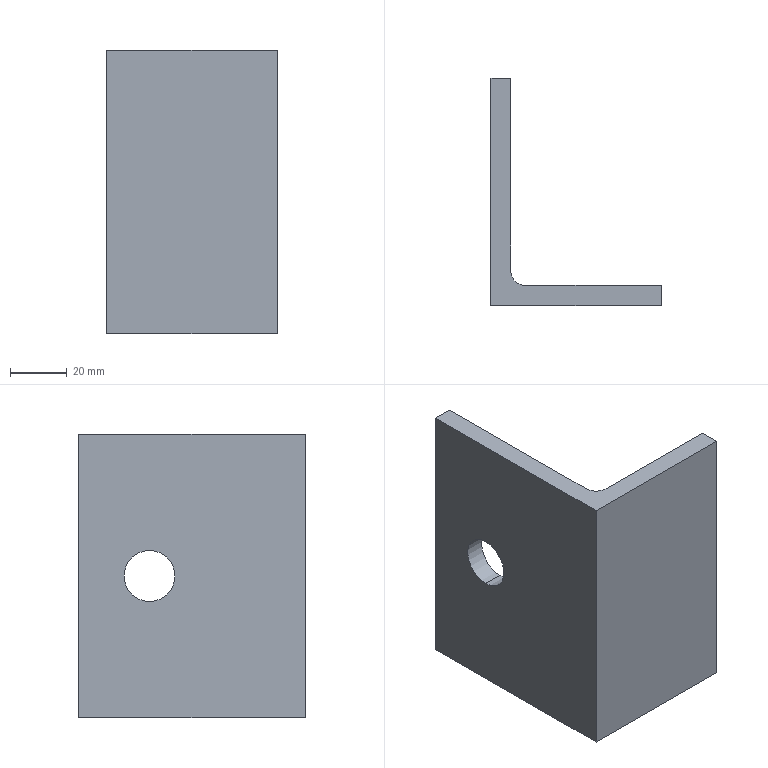Part | SolidWorks | features Extrusion 1, Fillet 1, ICE 1 | 1 solid | 11 faces | box 60 x 80 x 100 mm | volume 91855 mm3 | plane 8 | cylinder 3 | commonest cylinder face diameters 18 x2 10 x1
STEP:
#1=CARTESIAN_POINT('',(0.,-25.,59.));
#2=VERTEX_POINT('',#1);
#3=CARTESIAN_POINT('',(0.,-25.,41.));
#4=VERTEX_POINT('',#3);
#5=CARTESIAN_POINT('',(0.,-25.,50.));
#6=DIRECTION('',(1.,0.,0.));
#7=DIRECTION('',(0.,1.,0.));
#8=AXIS2_PLACEMENT_3D('',#5,#6,#7);
#9=CIRCLE('',#8,9.);
#10=EDGE_CURVE('',#2,#4,#9,.T.);
#11=ORIENTED_EDGE('',*,*,#10,.F.);
#12=CARTESIAN_POINT('',(7.,-25.,59.));
#13=VERTEX_POINT('',#12);
#14=CARTESIAN_POINT('',(-93.,-25.,59.));
#15=DIRECTION('',(1.,0.,0.));
#16=VECTOR('',#15,1000.);
#17=LINE('',#14,#16);
#18=EDGE_CURVE('',#2,#13,#17,.T.);
#19=ORIENTED_EDGE('',*,*,#18,.T.);
#20=CARTESIAN_POINT('',(7.,-25.,41.));
#21=VERTEX_POINT('',#20);
#22=CARTESIAN_POINT('',(7.,-25.,50.));
#23=DIRECTION('',(1.,0.,0.));
#24=DIRECTION('',(0.,0.,-1.));
#25=AXIS2_PLACEMENT_3D('',#22,#23,#24);
#26=CIRCLE('',#25,9.);
#27=EDGE_CURVE('',#13,#21,#26,.T.);
#28=ORIENTED_EDGE('',*,*,#27,.T.);
#29=CARTESIAN_POINT('',(-93.,-25.,41.));
#30=DIRECTION('',(1.,0.,0.));
#31=VECTOR('',#30,1000.);
#32=LINE('',#29,#31);
#33=EDGE_CURVE('',#4,#21,#32,.T.);
#34=ORIENTED_EDGE('',*,*,#33,.F.);
#35=EDGE_LOOP('',(#11,#19,#28,#34));
#36=FACE_OUTER_BOUND('',#35,.T.);
#37=CARTESIAN_POINT('',(-93.,-25.,50.));
#38=DIRECTION('',(1.,0.,0.));
#39=DIRECTION('',(0.,0.,-1.));
#40=AXIS2_PLACEMENT_3D('',#37,#38,#39);
#41=CYLINDRICAL_SURFACE('',#40,9.);
#42=ADVANCED_FACE('',(#36),#41,.F.);
#43=CARTESIAN_POINT('',(7.,0.,0.));
#44=VERTEX_POINT('',#43);
#45=CARTESIAN_POINT('',(0.,0.,0.));
#46=VERTEX_POINT('',#45);
#47=CARTESIAN_POINT('',(7.,0.,0.));
#48=DIRECTION('',(-1.,0.,0.));
#49=VECTOR('',#48,1000.);
#50=LINE('',#47,#49);
#51=EDGE_CURVE('',#44,#46,#50,.T.);
#52=ORIENTED_EDGE('',*,*,#51,.T.);
#53=CARTESIAN_POINT('',(0.,0.,100.));
#54=VERTEX_POINT('',#53);
#55=CARTESIAN_POINT('',(0.,0.,100.));
#56=DIRECTION('',(0.,0.,-1.));
#57=VECTOR('',#56,1000.);
#58=LINE('',#55,#57);
#59=EDGE_CURVE('',#54,#46,#58,.T.);
#60=ORIENTED_EDGE('',*,*,#59,.F.);
#61=CARTESIAN_POINT('',(7.,0.,100.));
#62=VERTEX_POINT('',#61);
#63=CARTESIAN_POINT('',(7.,0.,100.));
#64=DIRECTION('',(-1.,0.,0.));
#65=VECTOR('',#64,1000.);
#66=LINE('',#63,#65);
#67=EDGE_CURVE('',#62,#54,#66,.T.);
#68=ORIENTED_EDGE('',*,*,#67,.F.);
#69=CARTESIAN_POINT('',(7.,0.,100.));
#70=DIRECTION('',(0.,0.,-1.));
#71=VECTOR('',#70,1000.);
#72=LINE('',#69,#71);
#73=EDGE_CURVE('',#62,#44,#72,.T.);
#74=ORIENTED_EDGE('',*,*,#73,.T.);
#75=EDGE_LOOP('',(#52,#60,#68,#74));
#76=FACE_OUTER_BOUND('',#75,.T.);
#77=CARTESIAN_POINT('',(7.,0.,100.));
#78=DIRECTION('',(0.,-1.,0.));
#79=DIRECTION('',(0.,0.,-1.));
#80=AXIS2_PLACEMENT_3D('',#77,#78,#79);
#81=PLANE('',#80);
#82=ADVANCED_FACE('',(#76),#81,.F.);
#83=CARTESIAN_POINT('',(0.,-25.,50.));
#84=DIRECTION('',(1.,0.,0.));
#85=DIRECTION('',(0.,1.,0.));
#86=AXIS2_PLACEMENT_3D('',#83,#84,#85);
#87=CIRCLE('',#86,9.);
#88=EDGE_CURVE('',#4,#2,#87,.T.);
#89=ORIENTED_EDGE('',*,*,#88,.T.);
#90=ORIENTED_EDGE('',*,*,#10,.T.);
#91=EDGE_LOOP('',(#89,#90));
#92=FACE_BOUND('',#91,.T.);
#93=CARTESIAN_POINT('',(0.,-80.,0.));
#94=VERTEX_POINT('',#93);
#95=CARTESIAN_POINT('',(0.,0.,0.));
#96=DIRECTION('',(0.,-1.,0.));
#97=VECTOR('',#96,1000.);
#98=LINE('',#95,#97);
#99=EDGE_CURVE('',#46,#94,#98,.T.);
#100=ORIENTED_EDGE('',*,*,#99,.T.);
#101=CARTESIAN_POINT('',(0.,-80.,100.));
#102=VERTEX_POINT('',#101);
#103=CARTESIAN_POINT('',(0.,-80.,100.));
#104=DIRECTION('',(0.,0.,-1.));
#105=VECTOR('',#104,1000.);
#106=LINE('',#103,#105);
#107=EDGE_CURVE('',#102,#94,#106,.T.);
#108=ORIENTED_EDGE('',*,*,#107,.F.);
#109=CARTESIAN_POINT('',(0.,0.,100.));
#110=DIRECTION('',(0.,-1.,0.));
#111=VECTOR('',#110,1000.);
#112=LINE('',#109,#111);
#113=EDGE_CURVE('',#54,#102,#112,.T.);
#114=ORIENTED_EDGE('',*,*,#113,.F.);
#115=ORIENTED_EDGE('',*,*,#59,.T.);
#116=EDGE_LOOP('',(#100,#108,#114,#115));
#117=FACE_OUTER_BOUND('',#116,.T.);
#118=CARTESIAN_POINT('',(0.,0.,100.));
#119=DIRECTION('',(1.,0.,0.));
#120=DIRECTION('',(0.,1.,0.));
#121=AXIS2_PLACEMENT_3D('',#118,#119,#120);
#122=PLANE('',#121);
#123=ADVANCED_FACE('',(#92,#117),#122,.F.);
#124=CARTESIAN_POINT('',(60.,-80.,0.));
#125=VERTEX_POINT('',#124);
#126=CARTESIAN_POINT('',(0.,-80.,0.));
#127=DIRECTION('',(1.,0.,0.));
#128=VECTOR('',#127,1000.);
#129=LINE('',#126,#128);
#130=EDGE_CURVE('',#94,#125,#129,.T.);
#131=ORIENTED_EDGE('',*,*,#130,.T.);
#132=CARTESIAN_POINT('',(60.,-80.,100.));
#133=VERTEX_POINT('',#132);
#134=CARTESIAN_POINT('',(60.,-80.,100.));
#135=DIRECTION('',(0.,0.,-1.));
#136=VECTOR('',#135,1000.);
#137=LINE('',#134,#136);
#138=EDGE_CURVE('',#133,#125,#137,.T.);
#139=ORIENTED_EDGE('',*,*,#138,.F.);
#140=CARTESIAN_POINT('',(0.,-80.,100.));
#141=DIRECTION('',(1.,0.,0.));
#142=VECTOR('',#141,1000.);
#143=LINE('',#140,#142);
#144=EDGE_CURVE('',#102,#133,#143,.T.);
#145=ORIENTED_EDGE('',*,*,#144,.F.);
#146=ORIENTED_EDGE('',*,*,#107,.T.);
#147=EDGE_LOOP('',(#131,#139,#145,#146));
#148=FACE_OUTER_BOUND('',#147,.T.);
#149=CARTESIAN_POINT('',(0.,-80.,100.));
#150=DIRECTION('',(0.,1.,0.));
#151=DIRECTION('',(0.,0.,1.));
#152=AXIS2_PLACEMENT_3D('',#149,#150,#151);
#153=PLANE('',#152);
#154=ADVANCED_FACE('',(#148),#153,.F.);
#155=CARTESIAN_POINT('',(60.,-73.,0.));
#156=VERTEX_POINT('',#155);
#157=CARTESIAN_POINT('',(60.,-73.,0.));
#158=DIRECTION('',(0.,1.,0.));
#159=VECTOR('',#158,1000.);
#160=LINE('',#157,#159);
#161=EDGE_CURVE('',#125,#156,#160,.T.);
#162=ORIENTED_EDGE('',*,*,#161,.T.);
#163=CARTESIAN_POINT('',(60.,-73.,100.));
#164=VERTEX_POINT('',#163);
#165=CARTESIAN_POINT('',(60.,-73.,100.));
#166=DIRECTION('',(0.,0.,-1.));
#167=VECTOR('',#166,1000.);
#168=LINE('',#165,#167);
#169=EDGE_CURVE('',#164,#156,#168,.T.);
#170=ORIENTED_EDGE('',*,*,#169,.F.);
#171=CARTESIAN_POINT('',(60.,-73.,100.));
#172=DIRECTION('',(0.,1.,0.));
#173=VECTOR('',#172,1000.);
#174=LINE('',#171,#173);
#175=EDGE_CURVE('',#133,#164,#174,.T.);
#176=ORIENTED_EDGE('',*,*,#175,.F.);
#177=ORIENTED_EDGE('',*,*,#138,.T.);
#178=EDGE_LOOP('',(#162,#170,#176,#177));
#179=FACE_OUTER_BOUND('',#178,.T.);
#180=CARTESIAN_POINT('',(60.,-73.,100.));
#181=DIRECTION('',(-1.,0.,0.));
#182=DIRECTION('',(0.,0.,1.));
#183=AXIS2_PLACEMENT_3D('',#180,#181,#182);
#184=PLANE('',#183);
#185=ADVANCED_FACE('',(#179),#184,.F.);
#186=CARTESIAN_POINT('',(12.,-73.,0.));
#187=VERTEX_POINT('',#186);
#188=CARTESIAN_POINT('',(7.,-73.,0.));
#189=DIRECTION('',(-1.,0.,0.));
#190=VECTOR('',#189,1000.);
#191=LINE('',#188,#190);
#192=EDGE_CURVE('',#156,#187,#191,.T.);
#193=ORIENTED_EDGE('',*,*,#192,.T.);
#194=CARTESIAN_POINT('',(12.,-73.,100.));
#195=VERTEX_POINT('',#194);
#196=CARTESIAN_POINT('',(12.,-73.,100.));
#197=DIRECTION('',(0.,0.,1.));
#198=VECTOR('',#197,1000.);
#199=LINE('',#196,#198);
#200=EDGE_CURVE('',#187,#195,#199,.T.);
#201=ORIENTED_EDGE('',*,*,#200,.T.);
#202=CARTESIAN_POINT('',(7.,-73.,100.));
#203=DIRECTION('',(-1.,0.,0.));
#204=VECTOR('',#203,1000.);
#205=LINE('',#202,#204);
#206=EDGE_CURVE('',#164,#195,#205,.T.);
#207=ORIENTED_EDGE('',*,*,#206,.F.);
#208=ORIENTED_EDGE('',*,*,#169,.T.);
#209=EDGE_LOOP('',(#193,#201,#207,#208));
#210=FACE_OUTER_BOUND('',#209,.T.);
#211=CARTESIAN_POINT('',(7.,-73.,100.));
#212=DIRECTION('',(0.,-1.,0.));
#213=DIRECTION('',(0.,0.,-1.));
#214=AXIS2_PLACEMENT_3D('',#211,#212,#213);
#215=PLANE('',#214);
#216=ADVANCED_FACE('',(#210),#215,.F.);
#217=CARTESIAN_POINT('',(7.,-25.,50.));
#218=DIRECTION('',(1.,0.,0.));
#219=DIRECTION('',(0.,0.,-1.));
#220=AXIS2_PLACEMENT_3D('',#217,#218,#219);
#221=CIRCLE('',#220,9.);
#222=EDGE_CURVE('',#21,#13,#221,.T.);
#223=ORIENTED_EDGE('',*,*,#222,.F.);
#224=ORIENTED_EDGE('',*,*,#27,.F.);
#225=EDGE_LOOP('',(#223,#224));
#226=FACE_BOUND('',#225,.T.);
#227=CARTESIAN_POINT('',(7.,-68.,100.));
#228=VERTEX_POINT('',#227);
#229=CARTESIAN_POINT('',(7.,0.,100.));
#230=DIRECTION('',(0.,1.,0.));
#231=VECTOR('',#230,1000.);
#232=LINE('',#229,#231);
#233=EDGE_CURVE('',#228,#62,#232,.T.);
#234=ORIENTED_EDGE('',*,*,#233,.F.);
#235=CARTESIAN_POINT('',(7.,-68.,0.));
#236=VERTEX_POINT('',#235);
#237=CARTESIAN_POINT('',(7.,-68.,0.));
#238=DIRECTION('',(0.,0.,-1.));
#239=VECTOR('',#238,1000.);
#240=LINE('',#237,#239);
#241=EDGE_CURVE('',#228,#236,#240,.T.);
#242=ORIENTED_EDGE('',*,*,#241,.T.);
#243=CARTESIAN_POINT('',(7.,0.,0.));
#244=DIRECTION('',(0.,1.,0.));
#245=VECTOR('',#244,1000.);
#246=LINE('',#243,#245);
#247=EDGE_CURVE('',#236,#44,#246,.T.);
#248=ORIENTED_EDGE('',*,*,#247,.T.);
#249=ORIENTED_EDGE('',*,*,#73,.F.);
#250=EDGE_LOOP('',(#234,#242,#248,#249));
#251=FACE_OUTER_BOUND('',#250,.T.);
#252=CARTESIAN_POINT('',(7.,0.,100.));
#253=DIRECTION('',(-1.,0.,0.));
#254=DIRECTION('',(0.,0.,1.));
#255=AXIS2_PLACEMENT_3D('',#252,#253,#254);
#256=PLANE('',#255);
#257=ADVANCED_FACE('',(#226,#251),#256,.F.);
#258=ORIENTED_EDGE('',*,*,#67,.T.);
#259=ORIENTED_EDGE('',*,*,#113,.T.);
#260=ORIENTED_EDGE('',*,*,#144,.T.);
#261=ORIENTED_EDGE('',*,*,#175,.T.);
#262=ORIENTED_EDGE('',*,*,#206,.T.);
#263=CARTESIAN_POINT('',(12.,-68.,100.));
#264=DIRECTION('',(0.,0.,-1.));
#265=DIRECTION('',(1.,0.,0.));
#266=AXIS2_PLACEMENT_3D('',#263,#264,#265);
#267=CIRCLE('',#266,5.);
#268=EDGE_CURVE('',#195,#228,#267,.T.);
#269=ORIENTED_EDGE('',*,*,#268,.T.);
#270=ORIENTED_EDGE('',*,*,#233,.T.);
#271=EDGE_LOOP('',(#258,#259,#260,#261,#262,#269,#270));
#272=FACE_OUTER_BOUND('',#271,.T.);
#273=CARTESIAN_POINT('',(0.,0.,100.));
#274=DIRECTION('',(0.,0.,1.));
#275=DIRECTION('',(1.,0.,0.));
#276=AXIS2_PLACEMENT_3D('',#273,#274,#275);
#277=PLANE('',#276);
#278=ADVANCED_FACE('',(#272),#277,.T.);
#279=ORIENTED_EDGE('',*,*,#51,.F.);
#280=ORIENTED_EDGE('',*,*,#247,.F.);
#281=CARTESIAN_POINT('',(12.,-68.,0.));
#282=DIRECTION('',(0.,0.,1.));
#283=DIRECTION('',(1.,0.,0.));
#284=AXIS2_PLACEMENT_3D('',#281,#282,#283);
#285=CIRCLE('',#284,5.);
#286=EDGE_CURVE('',#236,#187,#285,.T.);
#287=ORIENTED_EDGE('',*,*,#286,.T.);
#288=ORIENTED_EDGE('',*,*,#192,.F.);
#289=ORIENTED_EDGE('',*,*,#161,.F.);
#290=ORIENTED_EDGE('',*,*,#130,.F.);
#291=ORIENTED_EDGE('',*,*,#99,.F.);
#292=EDGE_LOOP('',(#279,#280,#287,#288,#289,#290,#291));
#293=FACE_OUTER_BOUND('',#292,.T.);
#294=CARTESIAN_POINT('',(0.,0.,0.));
#295=DIRECTION('',(0.,0.,1.));
#296=DIRECTION('',(1.,0.,0.));
#297=AXIS2_PLACEMENT_3D('',#294,#295,#296);
#298=PLANE('',#297);
#299=ADVANCED_FACE('',(#293),#298,.F.);
#300=ORIENTED_EDGE('',*,*,#18,.F.);
#301=ORIENTED_EDGE('',*,*,#88,.F.);
#302=ORIENTED_EDGE('',*,*,#33,.T.);
#303=ORIENTED_EDGE('',*,*,#222,.T.);
#304=EDGE_LOOP('',(#300,#301,#302,#303));
#305=FACE_OUTER_BOUND('',#304,.T.);
#306=CARTESIAN_POINT('',(-93.,-25.,50.));
#307=DIRECTION('',(1.,0.,0.));
#308=DIRECTION('',(0.,0.,-1.));
#309=AXIS2_PLACEMENT_3D('',#306,#307,#308);
#310=CYLINDRICAL_SURFACE('',#309,9.);
#311=ADVANCED_FACE('',(#305),#310,.F.);
#312=ORIENTED_EDGE('',*,*,#268,.F.);
#313=ORIENTED_EDGE('',*,*,#200,.F.);
#314=ORIENTED_EDGE('',*,*,#286,.F.);
#315=ORIENTED_EDGE('',*,*,#241,.F.);
#316=EDGE_LOOP('',(#312,#313,#314,#315));
#317=FACE_OUTER_BOUND('',#316,.T.);
#318=CARTESIAN_POINT('',(12.,-68.,100.));
#319=DIRECTION('',(0.,0.,1.));
#320=DIRECTION('',(1.,0.,0.));
#321=AXIS2_PLACEMENT_3D('',#318,#319,#320);
#322=CYLINDRICAL_SURFACE('',#321,5.);
#323=ADVANCED_FACE('',(#317),#322,.F.);
#324=CLOSED_SHELL('',(#42,#82,#123,#154,#185,#216,#257,#278,#299,#311,#323));
#325=MANIFOLD_SOLID_BREP('',#324);
#326=CARTESIAN_POINT('',(0.,0.,0.));
#327=DIRECTION('',(0.,0.,1.));
#328=DIRECTION('',(1.,0.,0.));
#329=AXIS2_PLACEMENT_3D('',#326,#327,#328);
#330=(LENGTH_UNIT()NAMED_UNIT(*)SI_UNIT(.MILLI.,.METRE.));
#331=UNCERTAINTY_MEASURE_WITH_UNIT(LENGTH_MEASURE(0.00001),#330,'','');
#332=(NAMED_UNIT(*)PLANE_ANGLE_UNIT()SI_UNIT($,.RADIAN.));
#333=(NAMED_UNIT(*)SI_UNIT($,.STERADIAN.)SOLID_ANGLE_UNIT());
#334=(GEOMETRIC_REPRESENTATION_CONTEXT(3)GLOBAL_UNCERTAINTY_ASSIGNED_CONTEXT((#331))GLOBAL_UNIT_ASSIGNED_CONTEXT((#330,#332,#333))REPRESENTATION_CONTEXT('',''));
#335=ADVANCED_BREP_SHAPE_REPRESENTATION('',(#325,#329),#334);